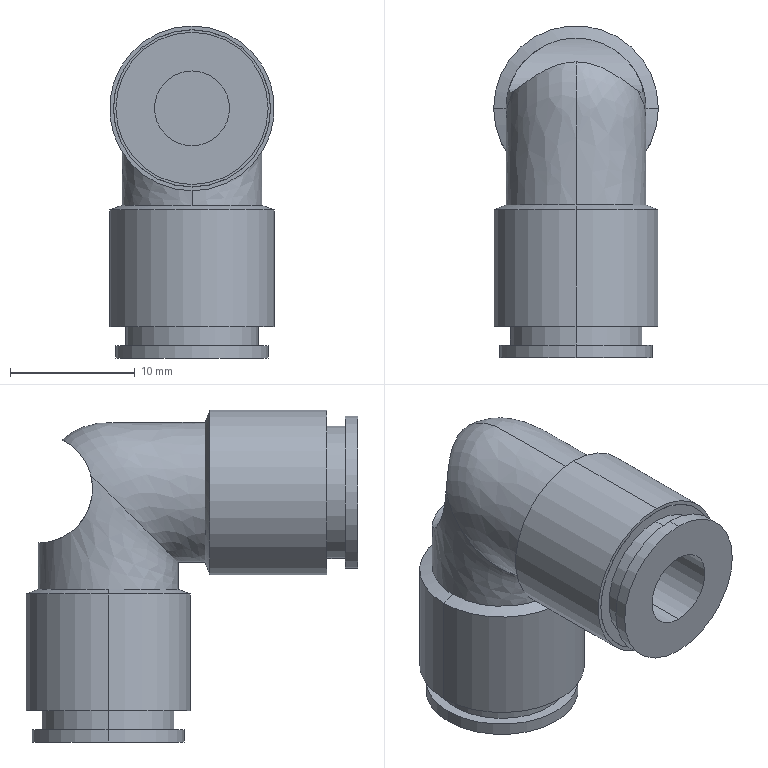Part | 1 solid | 51 faces | box 13.2 x 26.6 x 26.6 mm | volume 3731 mm3 | cylinder 29 | plane 14 | spline 4 | cone 4 | commonest cylinder face diameters 6 x4 10.6 x4 10.8 x4 12.2 x4 12.58 x4 12.6 x4